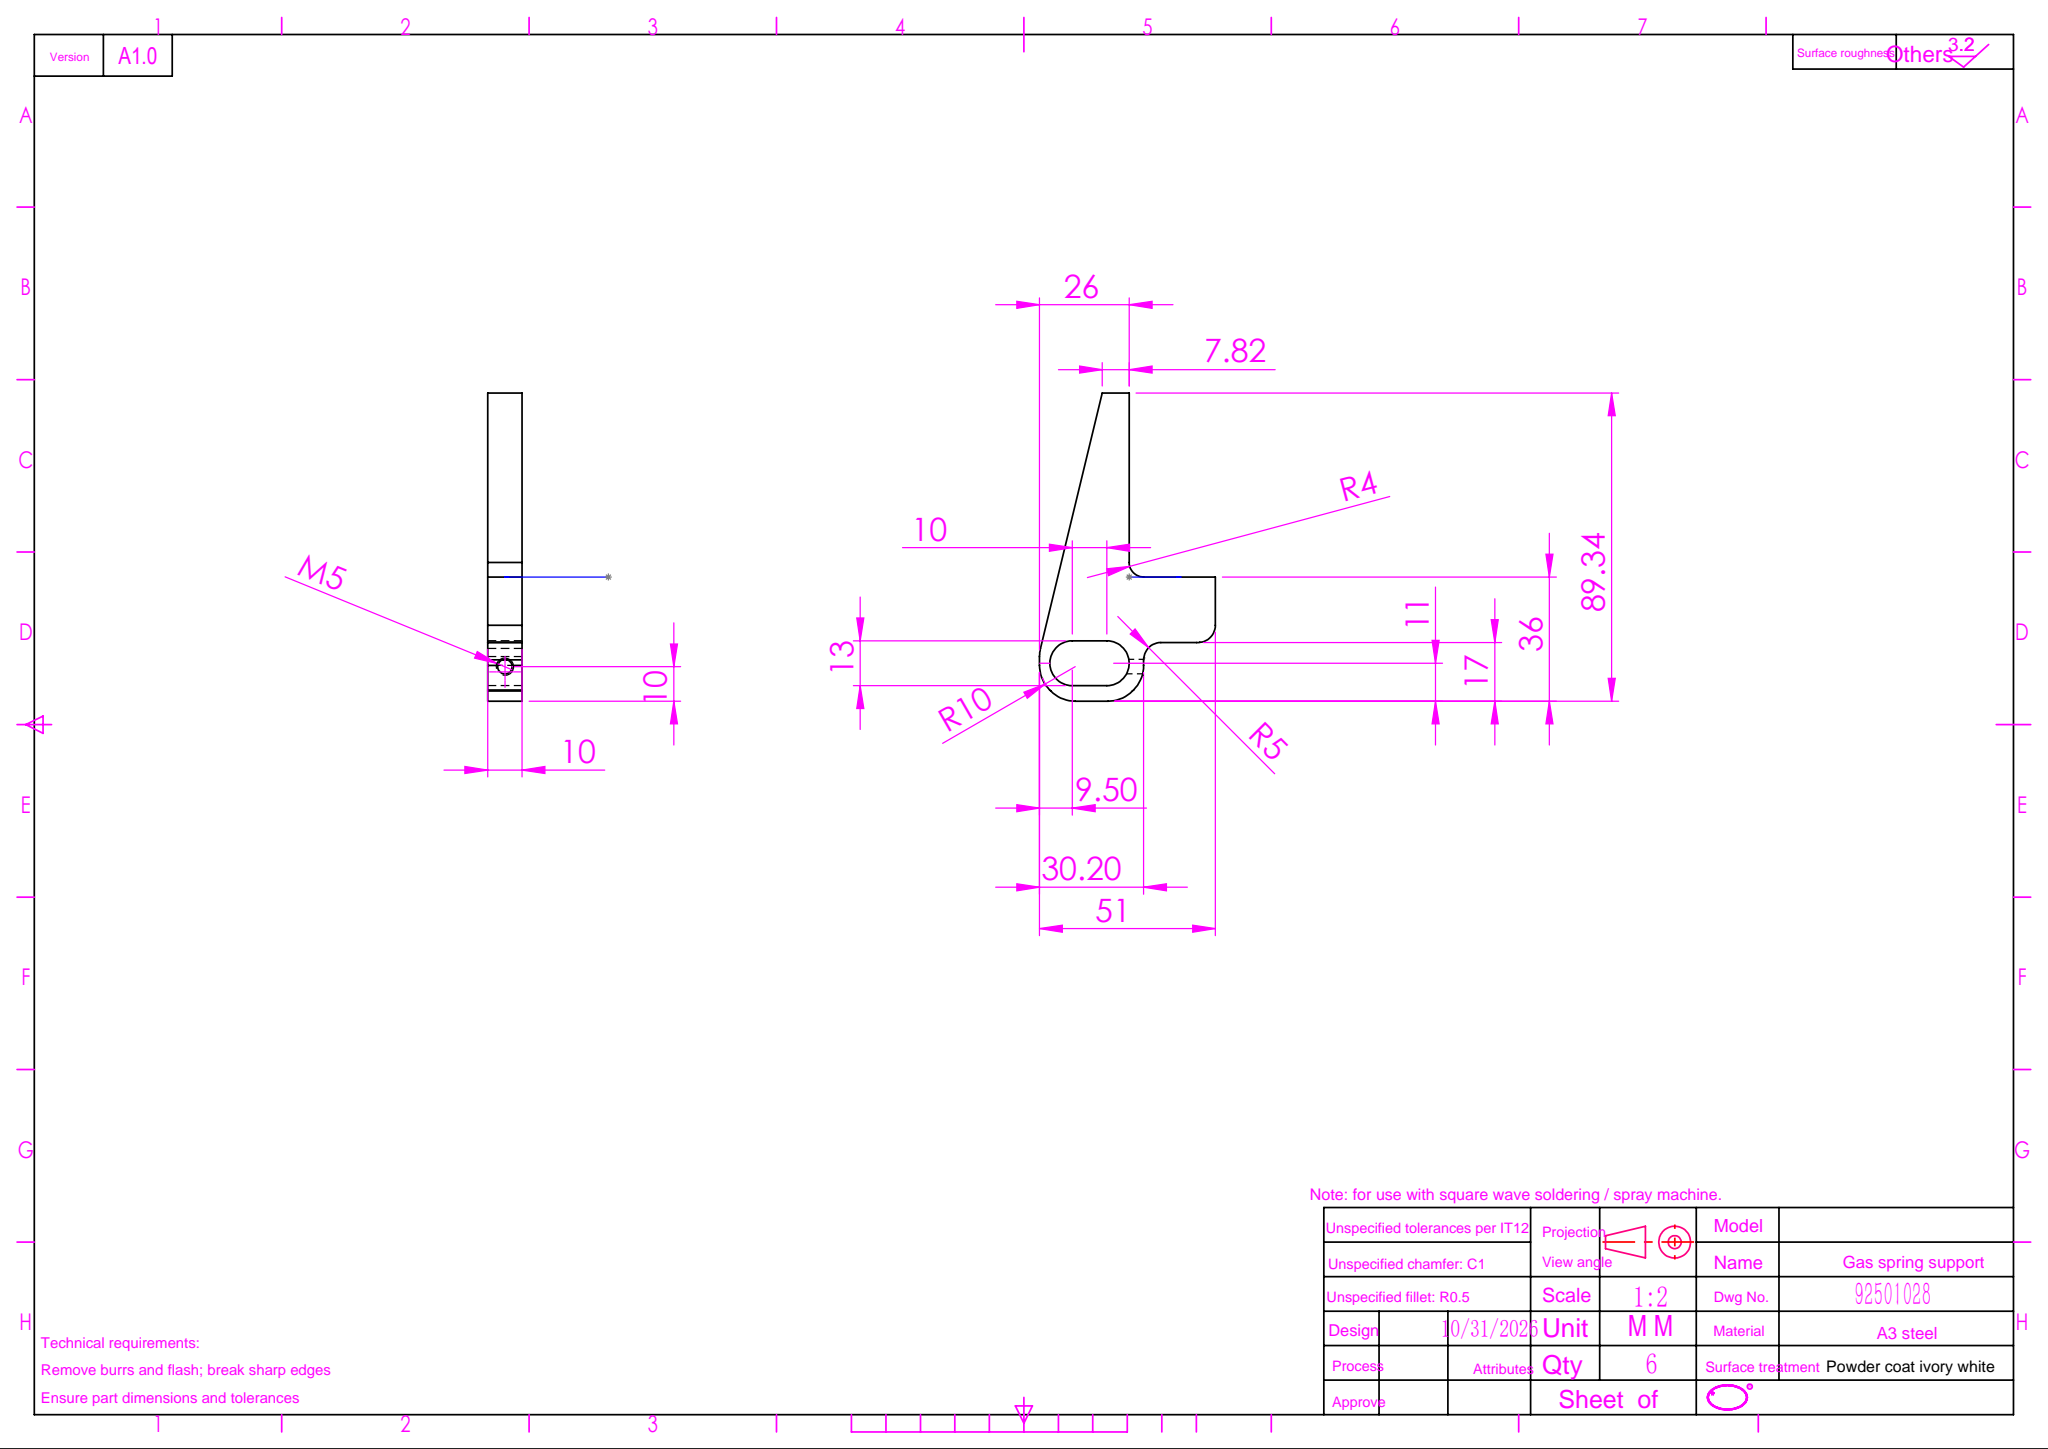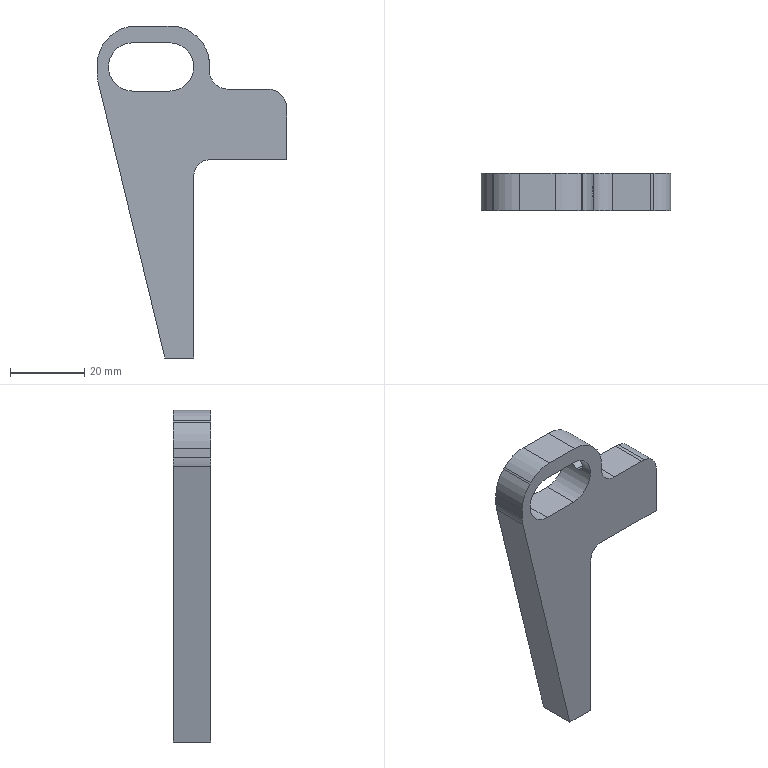Part | SolidWorks | features Fillet 4, ICE 4, MoveFace 2, SMBaseFlange 1, SheetMetal 1 | 1 solid | 30 faces | box 51 x 10 x 89.336 mm | volume 18730 mm3 | plane 17 | cylinder 13 | commonest cylinder face diameters 20 x6 4.2 x2 10 x2 13 x2 8.4 x1